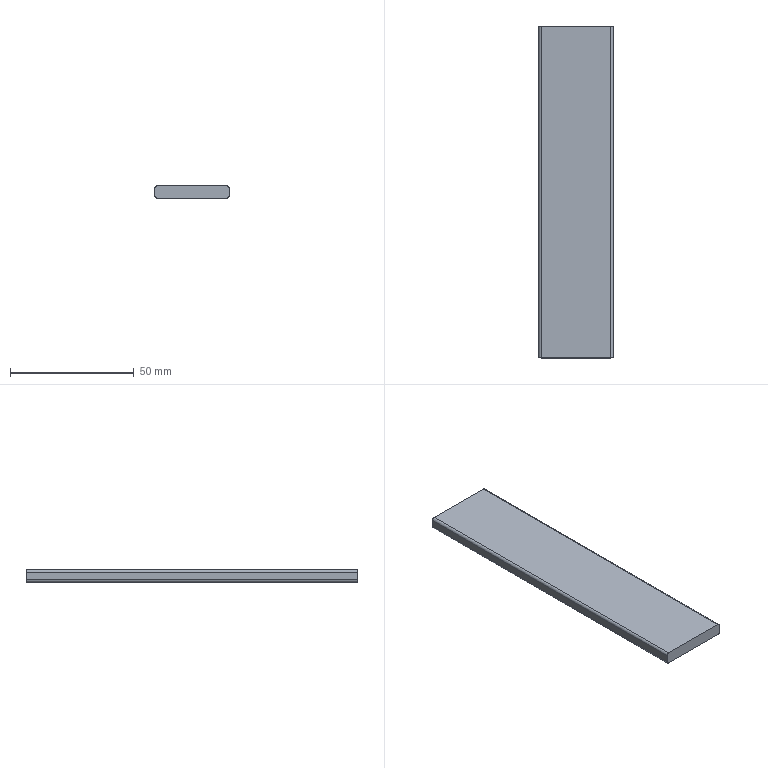Part | STEP file | Tube necking machine_id734_x_t | 1 solid | 10 faces | box 30 x 134 x 5 mm | volume 19985 mm3 | plane 6 | cylinder 4 | commonest cylinder face diameters 2 x4
STEP:
#1=CARTESIAN_POINT('',(0.,0.,0.));
#2=DIRECTION('',(0.,0.,1.));
#3=DIRECTION('',(1.,0.,0.));
#4=AXIS2_PLACEMENT_3D('',#1,#2,#3);
#5=CARTESIAN_POINT('',(-46.,-259.,196.));
#6=VERTEX_POINT('',#5);
#7=CARTESIAN_POINT('',(-74.,-259.,196.));
#8=VERTEX_POINT('',#7);
#9=CARTESIAN_POINT('',(-40.,-259.,196.));
#10=DIRECTION('',(-1.,0.,0.));
#11=VECTOR('',#10,1.);
#12=LINE('',#9,#11);
#13=CARTESIAN_POINT('',(-40.,-259.,196.));
#14=DIRECTION('',(0.,0.,-1.));
#15=DIRECTION('',(-1.,0.,0.));
#16=AXIS2_PLACEMENT_3D('',#13,#14,#15);
#17=PLANE('',#16);
#18=CARTESIAN_POINT('',(0.,0.));
#19=DIRECTION('',(1.,0.));
#20=VECTOR('',#19,1.);
#21=LINE('',#18,#20);
#22=(GEOMETRIC_REPRESENTATION_CONTEXT(2)PARAMETRIC_REPRESENTATION_CONTEXT()REPRESENTATION_CONTEXT('',''));
#23=DEFINITIONAL_REPRESENTATION('',(#21),#22);
#24=PCURVE('',#17,#23);
#25=CARTESIAN_POINT('',(0.,-259.,0.));
#26=DIRECTION('',(0.,-1.,0.));
#27=DIRECTION('',(0.,0.,-1.));
#28=AXIS2_PLACEMENT_3D('',#25,#26,#27);
#29=PLANE('',#28);
#30=CARTESIAN_POINT('',(-196.,-40.));
#31=DIRECTION('',(0.,-1.));
#32=VECTOR('',#31,1.);
#33=LINE('',#30,#32);
#34=(GEOMETRIC_REPRESENTATION_CONTEXT(2)PARAMETRIC_REPRESENTATION_CONTEXT()REPRESENTATION_CONTEXT('',''));
#35=DEFINITIONAL_REPRESENTATION('',(#33),#34);
#36=PCURVE('',#29,#35);
#37=SURFACE_CURVE('',#12,(#24,#36),.PCURVE_S1.);
#38=EDGE_CURVE('',#6,#8,#37,.T.);
#39=ORIENTED_EDGE('',*,*,#38,.F.);
#40=CARTESIAN_POINT('',(-46.,-125.,196.));
#41=VERTEX_POINT('',#40);
#42=CARTESIAN_POINT('',(-46.,-259.,196.));
#43=DIRECTION('',(0.,1.,0.));
#44=VECTOR('',#43,1.);
#45=LINE('',#42,#44);
#46=CARTESIAN_POINT('',(6.,0.));
#47=DIRECTION('',(0.,1.));
#48=VECTOR('',#47,1.);
#49=LINE('',#46,#48);
#50=(GEOMETRIC_REPRESENTATION_CONTEXT(2)PARAMETRIC_REPRESENTATION_CONTEXT()REPRESENTATION_CONTEXT('',''));
#51=DEFINITIONAL_REPRESENTATION('',(#49),#50);
#52=PCURVE('',#17,#51);
#53=CARTESIAN_POINT('',(-46.,-259.,195.));
#54=DIRECTION('',(0.,1.,0.));
#55=DIRECTION('',(0.,0.,1.));
#56=AXIS2_PLACEMENT_3D('',#53,#54,#55);
#57=CYLINDRICAL_SURFACE('',#56,1.);
#58=CARTESIAN_POINT('',(0.,0.));
#59=DIRECTION('',(0.,1.));
#60=VECTOR('',#59,1.);
#61=LINE('',#58,#60);
#62=(GEOMETRIC_REPRESENTATION_CONTEXT(2)PARAMETRIC_REPRESENTATION_CONTEXT()REPRESENTATION_CONTEXT('',''));
#63=DEFINITIONAL_REPRESENTATION('',(#61),#62);
#64=PCURVE('',#57,#63);
#65=SURFACE_CURVE('',#45,(#52,#64),.PCURVE_S1.);
#66=EDGE_CURVE('',#6,#41,#65,.T.);
#67=ORIENTED_EDGE('',*,*,#66,.T.);
#68=CARTESIAN_POINT('',(-74.,-125.,196.));
#69=VERTEX_POINT('',#68);
#70=CARTESIAN_POINT('',(-40.,-125.,196.));
#71=DIRECTION('',(-1.,0.,0.));
#72=VECTOR('',#71,1.);
#73=LINE('',#70,#72);
#74=CARTESIAN_POINT('',(0.,134.));
#75=DIRECTION('',(1.,0.));
#76=VECTOR('',#75,1.);
#77=LINE('',#74,#76);
#78=(GEOMETRIC_REPRESENTATION_CONTEXT(2)PARAMETRIC_REPRESENTATION_CONTEXT()REPRESENTATION_CONTEXT('',''));
#79=DEFINITIONAL_REPRESENTATION('',(#77),#78);
#80=PCURVE('',#17,#79);
#81=CARTESIAN_POINT('',(0.,-125.,0.));
#82=DIRECTION('',(0.,-1.,0.));
#83=DIRECTION('',(0.,0.,-1.));
#84=AXIS2_PLACEMENT_3D('',#81,#82,#83);
#85=PLANE('',#84);
#86=CARTESIAN_POINT('',(-196.,-40.));
#87=DIRECTION('',(0.,-1.));
#88=VECTOR('',#87,1.);
#89=LINE('',#86,#88);
#90=(GEOMETRIC_REPRESENTATION_CONTEXT(2)PARAMETRIC_REPRESENTATION_CONTEXT()REPRESENTATION_CONTEXT('',''));
#91=DEFINITIONAL_REPRESENTATION('',(#89),#90);
#92=PCURVE('',#85,#91);
#93=SURFACE_CURVE('',#73,(#80,#92),.PCURVE_S1.);
#94=EDGE_CURVE('',#41,#69,#93,.T.);
#95=ORIENTED_EDGE('',*,*,#94,.T.);
#96=CARTESIAN_POINT('',(-74.,-259.,196.));
#97=DIRECTION('',(0.,-1.,0.));
#98=VECTOR('',#97,1.);
#99=LINE('',#96,#98);
#100=CARTESIAN_POINT('',(34.,0.));
#101=DIRECTION('',(0.,-1.));
#102=VECTOR('',#101,1.);
#103=LINE('',#100,#102);
#104=(GEOMETRIC_REPRESENTATION_CONTEXT(2)PARAMETRIC_REPRESENTATION_CONTEXT()REPRESENTATION_CONTEXT('',''));
#105=DEFINITIONAL_REPRESENTATION('',(#103),#104);
#106=PCURVE('',#17,#105);
#107=CARTESIAN_POINT('',(-74.,-259.,195.));
#108=DIRECTION('',(0.,1.,0.));
#109=DIRECTION('',(0.,0.,1.));
#110=AXIS2_PLACEMENT_3D('',#107,#108,#109);
#111=CYLINDRICAL_SURFACE('',#110,1.);
#112=CARTESIAN_POINT('',(6.283,0.));
#113=DIRECTION('',(0.,-1.));
#114=VECTOR('',#113,1.);
#115=LINE('',#112,#114);
#116=(GEOMETRIC_REPRESENTATION_CONTEXT(2)PARAMETRIC_REPRESENTATION_CONTEXT()REPRESENTATION_CONTEXT('',''));
#117=DEFINITIONAL_REPRESENTATION('',(#115),#116);
#118=PCURVE('',#111,#117);
#119=SURFACE_CURVE('',#99,(#106,#118),.PCURVE_S1.);
#120=EDGE_CURVE('',#69,#8,#119,.T.);
#121=ORIENTED_EDGE('',*,*,#120,.T.);
#122=EDGE_LOOP('',(#39,#67,#95,#121));
#123=FACE_BOUND('',#122,.T.);
#124=ADVANCED_FACE('',(#123),#17,.F.);
#125=CARTESIAN_POINT('',(-75.,-125.,195.));
#126=VERTEX_POINT('',#125);
#127=CARTESIAN_POINT('',(-75.,-125.,192.));
#128=VERTEX_POINT('',#127);
#129=CARTESIAN_POINT('',(-75.,-125.,196.));
#130=DIRECTION('',(0.,0.,-1.));
#131=VECTOR('',#130,1.);
#132=LINE('',#129,#131);
#133=CARTESIAN_POINT('',(-75.,-259.,196.));
#134=DIRECTION('',(1.,0.,0.));
#135=DIRECTION('',(0.,0.,-1.));
#136=AXIS2_PLACEMENT_3D('',#133,#134,#135);
#137=PLANE('',#136);
#138=CARTESIAN_POINT('',(0.,134.));
#139=DIRECTION('',(1.,0.));
#140=VECTOR('',#139,1.);
#141=LINE('',#138,#140);
#142=(GEOMETRIC_REPRESENTATION_CONTEXT(2)PARAMETRIC_REPRESENTATION_CONTEXT()REPRESENTATION_CONTEXT('',''));
#143=DEFINITIONAL_REPRESENTATION('',(#141),#142);
#144=PCURVE('',#137,#143);
#145=CARTESIAN_POINT('',(-196.,-75.));
#146=DIRECTION('',(1.,0.));
#147=VECTOR('',#146,1.);
#148=LINE('',#145,#147);
#149=(GEOMETRIC_REPRESENTATION_CONTEXT(2)PARAMETRIC_REPRESENTATION_CONTEXT()REPRESENTATION_CONTEXT('',''));
#150=DEFINITIONAL_REPRESENTATION('',(#148),#149);
#151=PCURVE('',#85,#150);
#152=SURFACE_CURVE('',#132,(#144,#151),.PCURVE_S1.);
#153=EDGE_CURVE('',#126,#128,#152,.T.);
#154=ORIENTED_EDGE('',*,*,#153,.T.);
#155=CARTESIAN_POINT('',(-75.,-259.,192.));
#156=VERTEX_POINT('',#155);
#157=CARTESIAN_POINT('',(-75.,-259.,192.));
#158=DIRECTION('',(0.,-1.,0.));
#159=VECTOR('',#158,1.);
#160=LINE('',#157,#159);
#161=CARTESIAN_POINT('',(4.,0.));
#162=DIRECTION('',(0.,-1.));
#163=VECTOR('',#162,1.);
#164=LINE('',#161,#163);
#165=(GEOMETRIC_REPRESENTATION_CONTEXT(2)PARAMETRIC_REPRESENTATION_CONTEXT()REPRESENTATION_CONTEXT('',''));
#166=DEFINITIONAL_REPRESENTATION('',(#164),#165);
#167=PCURVE('',#137,#166);
#168=CARTESIAN_POINT('',(-74.,-259.,192.));
#169=DIRECTION('',(0.,1.,0.));
#170=DIRECTION('',(0.,0.,1.));
#171=AXIS2_PLACEMENT_3D('',#168,#169,#170);
#172=CYLINDRICAL_SURFACE('',#171,1.);
#173=CARTESIAN_POINT('',(4.712,0.));
#174=DIRECTION('',(0.,-1.));
#175=VECTOR('',#174,1.);
#176=LINE('',#173,#175);
#177=(GEOMETRIC_REPRESENTATION_CONTEXT(2)PARAMETRIC_REPRESENTATION_CONTEXT()REPRESENTATION_CONTEXT('',''));
#178=DEFINITIONAL_REPRESENTATION('',(#176),#177);
#179=PCURVE('',#172,#178);
#180=SURFACE_CURVE('',#160,(#167,#179),.PCURVE_S1.);
#181=EDGE_CURVE('',#128,#156,#180,.T.);
#182=ORIENTED_EDGE('',*,*,#181,.T.);
#183=CARTESIAN_POINT('',(-75.,-259.,195.));
#184=VERTEX_POINT('',#183);
#185=CARTESIAN_POINT('',(-75.,-259.,196.));
#186=DIRECTION('',(0.,0.,-1.));
#187=VECTOR('',#186,1.);
#188=LINE('',#185,#187);
#189=CARTESIAN_POINT('',(0.,0.));
#190=DIRECTION('',(1.,0.));
#191=VECTOR('',#190,1.);
#192=LINE('',#189,#191);
#193=(GEOMETRIC_REPRESENTATION_CONTEXT(2)PARAMETRIC_REPRESENTATION_CONTEXT()REPRESENTATION_CONTEXT('',''));
#194=DEFINITIONAL_REPRESENTATION('',(#192),#193);
#195=PCURVE('',#137,#194);
#196=CARTESIAN_POINT('',(-196.,-75.));
#197=DIRECTION('',(1.,0.));
#198=VECTOR('',#197,1.);
#199=LINE('',#196,#198);
#200=(GEOMETRIC_REPRESENTATION_CONTEXT(2)PARAMETRIC_REPRESENTATION_CONTEXT()REPRESENTATION_CONTEXT('',''));
#201=DEFINITIONAL_REPRESENTATION('',(#199),#200);
#202=PCURVE('',#29,#201);
#203=SURFACE_CURVE('',#188,(#195,#202),.PCURVE_S1.);
#204=EDGE_CURVE('',#184,#156,#203,.T.);
#205=ORIENTED_EDGE('',*,*,#204,.F.);
#206=CARTESIAN_POINT('',(-75.,-259.,195.));
#207=DIRECTION('',(0.,1.,0.));
#208=VECTOR('',#207,1.);
#209=LINE('',#206,#208);
#210=CARTESIAN_POINT('',(1.,0.));
#211=DIRECTION('',(0.,1.));
#212=VECTOR('',#211,1.);
#213=LINE('',#210,#212);
#214=(GEOMETRIC_REPRESENTATION_CONTEXT(2)PARAMETRIC_REPRESENTATION_CONTEXT()REPRESENTATION_CONTEXT('',''));
#215=DEFINITIONAL_REPRESENTATION('',(#213),#214);
#216=PCURVE('',#137,#215);
#217=CARTESIAN_POINT('',(4.712,0.));
#218=DIRECTION('',(0.,1.));
#219=VECTOR('',#218,1.);
#220=LINE('',#217,#219);
#221=(GEOMETRIC_REPRESENTATION_CONTEXT(2)PARAMETRIC_REPRESENTATION_CONTEXT()REPRESENTATION_CONTEXT('',''));
#222=DEFINITIONAL_REPRESENTATION('',(#220),#221);
#223=PCURVE('',#111,#222);
#224=SURFACE_CURVE('',#209,(#216,#223),.PCURVE_S1.);
#225=EDGE_CURVE('',#184,#126,#224,.T.);
#226=ORIENTED_EDGE('',*,*,#225,.T.);
#227=EDGE_LOOP('',(#154,#182,#205,#226));
#228=FACE_BOUND('',#227,.T.);
#229=ADVANCED_FACE('',(#228),#137,.F.);
#230=CARTESIAN_POINT('',(-74.,-125.,191.));
#231=VERTEX_POINT('',#230);
#232=CARTESIAN_POINT('',(-46.,-125.,191.));
#233=VERTEX_POINT('',#232);
#234=CARTESIAN_POINT('',(-75.,-125.,191.));
#235=DIRECTION('',(1.,0.,0.));
#236=VECTOR('',#235,1.);
#237=LINE('',#234,#236);
#238=CARTESIAN_POINT('',(-75.,-259.,191.));
#239=DIRECTION('',(0.,0.,1.));
#240=DIRECTION('',(1.,0.,0.));
#241=AXIS2_PLACEMENT_3D('',#238,#239,#240);
#242=PLANE('',#241);
#243=CARTESIAN_POINT('',(0.,134.));
#244=DIRECTION('',(1.,0.));
#245=VECTOR('',#244,1.);
#246=LINE('',#243,#245);
#247=(GEOMETRIC_REPRESENTATION_CONTEXT(2)PARAMETRIC_REPRESENTATION_CONTEXT()REPRESENTATION_CONTEXT('',''));
#248=DEFINITIONAL_REPRESENTATION('',(#246),#247);
#249=PCURVE('',#242,#248);
#250=CARTESIAN_POINT('',(-191.,-75.));
#251=DIRECTION('',(0.,1.));
#252=VECTOR('',#251,1.);
#253=LINE('',#250,#252);
#254=(GEOMETRIC_REPRESENTATION_CONTEXT(2)PARAMETRIC_REPRESENTATION_CONTEXT()REPRESENTATION_CONTEXT('',''));
#255=DEFINITIONAL_REPRESENTATION('',(#253),#254);
#256=PCURVE('',#85,#255);
#257=SURFACE_CURVE('',#237,(#249,#256),.PCURVE_S1.);
#258=EDGE_CURVE('',#231,#233,#257,.T.);
#259=ORIENTED_EDGE('',*,*,#258,.T.);
#260=CARTESIAN_POINT('',(-46.,-259.,191.));
#261=VERTEX_POINT('',#260);
#262=CARTESIAN_POINT('',(-46.,-259.,191.));
#263=DIRECTION('',(0.,-1.,0.));
#264=VECTOR('',#263,1.);
#265=LINE('',#262,#264);
#266=CARTESIAN_POINT('',(29.,0.));
#267=DIRECTION('',(0.,-1.));
#268=VECTOR('',#267,1.);
#269=LINE('',#266,#268);
#270=(GEOMETRIC_REPRESENTATION_CONTEXT(2)PARAMETRIC_REPRESENTATION_CONTEXT()REPRESENTATION_CONTEXT('',''));
#271=DEFINITIONAL_REPRESENTATION('',(#269),#270);
#272=PCURVE('',#242,#271);
#273=CARTESIAN_POINT('',(-46.,-259.,192.));
#274=DIRECTION('',(0.,1.,0.));
#275=DIRECTION('',(0.,0.,1.));
#276=AXIS2_PLACEMENT_3D('',#273,#274,#275);
#277=CYLINDRICAL_SURFACE('',#276,1.);
#278=CARTESIAN_POINT('',(3.142,0.));
#279=DIRECTION('',(0.,-1.));
#280=VECTOR('',#279,1.);
#281=LINE('',#278,#280);
#282=(GEOMETRIC_REPRESENTATION_CONTEXT(2)PARAMETRIC_REPRESENTATION_CONTEXT()REPRESENTATION_CONTEXT('',''));
#283=DEFINITIONAL_REPRESENTATION('',(#281),#282);
#284=PCURVE('',#277,#283);
#285=SURFACE_CURVE('',#265,(#272,#284),.PCURVE_S1.);
#286=EDGE_CURVE('',#233,#261,#285,.T.);
#287=ORIENTED_EDGE('',*,*,#286,.T.);
#288=CARTESIAN_POINT('',(-74.,-259.,191.));
#289=VERTEX_POINT('',#288);
#290=CARTESIAN_POINT('',(-75.,-259.,191.));
#291=DIRECTION('',(1.,0.,0.));
#292=VECTOR('',#291,1.);
#293=LINE('',#290,#292);
#294=CARTESIAN_POINT('',(0.,0.));
#295=DIRECTION('',(1.,0.));
#296=VECTOR('',#295,1.);
#297=LINE('',#294,#296);
#298=(GEOMETRIC_REPRESENTATION_CONTEXT(2)PARAMETRIC_REPRESENTATION_CONTEXT()REPRESENTATION_CONTEXT('',''));
#299=DEFINITIONAL_REPRESENTATION('',(#297),#298);
#300=PCURVE('',#242,#299);
#301=CARTESIAN_POINT('',(-191.,-75.));
#302=DIRECTION('',(0.,1.));
#303=VECTOR('',#302,1.);
#304=LINE('',#301,#303);
#305=(GEOMETRIC_REPRESENTATION_CONTEXT(2)PARAMETRIC_REPRESENTATION_CONTEXT()REPRESENTATION_CONTEXT('',''));
#306=DEFINITIONAL_REPRESENTATION('',(#304),#305);
#307=PCURVE('',#29,#306);
#308=SURFACE_CURVE('',#293,(#300,#307),.PCURVE_S1.);
#309=EDGE_CURVE('',#289,#261,#308,.T.);
#310=ORIENTED_EDGE('',*,*,#309,.F.);
#311=CARTESIAN_POINT('',(-74.,-259.,191.));
#312=DIRECTION('',(0.,1.,0.));
#313=VECTOR('',#312,1.);
#314=LINE('',#311,#313);
#315=CARTESIAN_POINT('',(1.,0.));
#316=DIRECTION('',(0.,1.));
#317=VECTOR('',#316,1.);
#318=LINE('',#315,#317);
#319=(GEOMETRIC_REPRESENTATION_CONTEXT(2)PARAMETRIC_REPRESENTATION_CONTEXT()REPRESENTATION_CONTEXT('',''));
#320=DEFINITIONAL_REPRESENTATION('',(#318),#319);
#321=PCURVE('',#242,#320);
#322=CARTESIAN_POINT('',(3.142,0.));
#323=DIRECTION('',(0.,1.));
#324=VECTOR('',#323,1.);
#325=LINE('',#322,#324);
#326=(GEOMETRIC_REPRESENTATION_CONTEXT(2)PARAMETRIC_REPRESENTATION_CONTEXT()REPRESENTATION_CONTEXT('',''));
#327=DEFINITIONAL_REPRESENTATION('',(#325),#326);
#328=PCURVE('',#172,#327);
#329=SURFACE_CURVE('',#314,(#321,#328),.PCURVE_S1.);
#330=EDGE_CURVE('',#289,#231,#329,.T.);
#331=ORIENTED_EDGE('',*,*,#330,.T.);
#332=EDGE_LOOP('',(#259,#287,#310,#331));
#333=FACE_BOUND('',#332,.T.);
#334=ADVANCED_FACE('',(#333),#242,.F.);
#335=CARTESIAN_POINT('',(-45.,-259.,192.));
#336=VERTEX_POINT('',#335);
#337=CARTESIAN_POINT('',(-45.,-259.,195.));
#338=VERTEX_POINT('',#337);
#339=CARTESIAN_POINT('',(-45.,-259.,191.));
#340=DIRECTION('',(0.,0.,1.));
#341=VECTOR('',#340,1.);
#342=LINE('',#339,#341);
#343=CARTESIAN_POINT('',(-45.,-259.,191.));
#344=DIRECTION('',(-1.,0.,0.));
#345=DIRECTION('',(0.,0.,1.));
#346=AXIS2_PLACEMENT_3D('',#343,#344,#345);
#347=PLANE('',#346);
#348=CARTESIAN_POINT('',(0.,0.));
#349=DIRECTION('',(1.,0.));
#350=VECTOR('',#349,1.);
#351=LINE('',#348,#350);
#352=(GEOMETRIC_REPRESENTATION_CONTEXT(2)PARAMETRIC_REPRESENTATION_CONTEXT()REPRESENTATION_CONTEXT('',''));
#353=DEFINITIONAL_REPRESENTATION('',(#351),#352);
#354=PCURVE('',#347,#353);
#355=CARTESIAN_POINT('',(-191.,-45.));
#356=DIRECTION('',(-1.,0.));
#357=VECTOR('',#356,1.);
#358=LINE('',#355,#357);
#359=(GEOMETRIC_REPRESENTATION_CONTEXT(2)PARAMETRIC_REPRESENTATION_CONTEXT()REPRESENTATION_CONTEXT('',''));
#360=DEFINITIONAL_REPRESENTATION('',(#358),#359);
#361=PCURVE('',#29,#360);
#362=SURFACE_CURVE('',#342,(#354,#361),.PCURVE_S1.);
#363=EDGE_CURVE('',#336,#338,#362,.T.);
#364=ORIENTED_EDGE('',*,*,#363,.F.);
#365=CARTESIAN_POINT('',(-45.,-125.,192.));
#366=VERTEX_POINT('',#365);
#367=CARTESIAN_POINT('',(-45.,-259.,192.));
#368=DIRECTION('',(0.,1.,0.));
#369=VECTOR('',#368,1.);
#370=LINE('',#367,#369);
#371=CARTESIAN_POINT('',(1.,0.));
#372=DIRECTION('',(0.,1.));
#373=VECTOR('',#372,1.);
#374=LINE('',#371,#373);
#375=(GEOMETRIC_REPRESENTATION_CONTEXT(2)PARAMETRIC_REPRESENTATION_CONTEXT()REPRESENTATION_CONTEXT('',''));
#376=DEFINITIONAL_REPRESENTATION('',(#374),#375);
#377=PCURVE('',#347,#376);
#378=CARTESIAN_POINT('',(1.571,0.));
#379=DIRECTION('',(0.,1.));
#380=VECTOR('',#379,1.);
#381=LINE('',#378,#380);
#382=(GEOMETRIC_REPRESENTATION_CONTEXT(2)PARAMETRIC_REPRESENTATION_CONTEXT()REPRESENTATION_CONTEXT('',''));
#383=DEFINITIONAL_REPRESENTATION('',(#381),#382);
#384=PCURVE('',#277,#383);
#385=SURFACE_CURVE('',#370,(#377,#384),.PCURVE_S1.);
#386=EDGE_CURVE('',#336,#366,#385,.T.);
#387=ORIENTED_EDGE('',*,*,#386,.T.);
#388=CARTESIAN_POINT('',(-45.,-125.,195.));
#389=VERTEX_POINT('',#388);
#390=CARTESIAN_POINT('',(-45.,-125.,191.));
#391=DIRECTION('',(0.,0.,1.));
#392=VECTOR('',#391,1.);
#393=LINE('',#390,#392);
#394=CARTESIAN_POINT('',(0.,134.));
#395=DIRECTION('',(1.,0.));
#396=VECTOR('',#395,1.);
#397=LINE('',#394,#396);
#398=(GEOMETRIC_REPRESENTATION_CONTEXT(2)PARAMETRIC_REPRESENTATION_CONTEXT()REPRESENTATION_CONTEXT('',''));
#399=DEFINITIONAL_REPRESENTATION('',(#397),#398);
#400=PCURVE('',#347,#399);
#401=CARTESIAN_POINT('',(-191.,-45.));
#402=DIRECTION('',(-1.,0.));
#403=VECTOR('',#402,1.);
#404=LINE('',#401,#403);
#405=(GEOMETRIC_REPRESENTATION_CONTEXT(2)PARAMETRIC_REPRESENTATION_CONTEXT()REPRESENTATION_CONTEXT('',''));
#406=DEFINITIONAL_REPRESENTATION('',(#404),#405);
#407=PCURVE('',#85,#406);
#408=SURFACE_CURVE('',#393,(#400,#407),.PCURVE_S1.);
#409=EDGE_CURVE('',#366,#389,#408,.T.);
#410=ORIENTED_EDGE('',*,*,#409,.T.);
#411=CARTESIAN_POINT('',(-45.,-259.,195.));
#412=DIRECTION('',(0.,-1.,0.));
#413=VECTOR('',#412,1.);
#414=LINE('',#411,#413);
#415=CARTESIAN_POINT('',(4.,0.));
#416=DIRECTION('',(0.,-1.));
#417=VECTOR('',#416,1.);
#418=LINE('',#415,#417);
#419=(GEOMETRIC_REPRESENTATION_CONTEXT(2)PARAMETRIC_REPRESENTATION_CONTEXT()REPRESENTATION_CONTEXT('',''));
#420=DEFINITIONAL_REPRESENTATION('',(#418),#419);
#421=PCURVE('',#347,#420);
#422=CARTESIAN_POINT('',(1.571,0.));
#423=DIRECTION('',(0.,-1.));
#424=VECTOR('',#423,1.);
#425=LINE('',#422,#424);
#426=(GEOMETRIC_REPRESENTATION_CONTEXT(2)PARAMETRIC_REPRESENTATION_CONTEXT()REPRESENTATION_CONTEXT('',''));
#427=DEFINITIONAL_REPRESENTATION('',(#425),#426);
#428=PCURVE('',#57,#427);
#429=SURFACE_CURVE('',#414,(#421,#428),.PCURVE_S1.);
#430=EDGE_CURVE('',#389,#338,#429,.T.);
#431=ORIENTED_EDGE('',*,*,#430,.T.);
#432=EDGE_LOOP('',(#364,#387,#410,#431));
#433=FACE_BOUND('',#432,.T.);
#434=ADVANCED_FACE('',(#433),#347,.F.);
#435=ORIENTED_EDGE('',*,*,#309,.T.);
#436=CARTESIAN_POINT('',(-46.,-259.,192.));
#437=DIRECTION('',(0.,-1.,0.));
#438=DIRECTION('',(0.,0.,-1.));
#439=AXIS2_PLACEMENT_3D('',#436,#437,#438);
#440=CIRCLE('',#439,1.);
#441=CARTESIAN_POINT('',(-192.,-46.));
#442=DIRECTION('',(1.,0.));
#443=AXIS2_PLACEMENT_2D('',#441,#442);
#444=CIRCLE('',#443,1.);
#445=(GEOMETRIC_REPRESENTATION_CONTEXT(2)PARAMETRIC_REPRESENTATION_CONTEXT()REPRESENTATION_CONTEXT('',''));
#446=DEFINITIONAL_REPRESENTATION('',(#444),#445);
#447=PCURVE('',#29,#446);
#448=CARTESIAN_POINT('',(3.142,0.));
#449=DIRECTION('',(-1.,0.));
#450=VECTOR('',#449,1.);
#451=LINE('',#448,#450);
#452=(GEOMETRIC_REPRESENTATION_CONTEXT(2)PARAMETRIC_REPRESENTATION_CONTEXT()REPRESENTATION_CONTEXT('',''));
#453=DEFINITIONAL_REPRESENTATION('',(#451),#452);
#454=PCURVE('',#277,#453);
#455=SURFACE_CURVE('',#440,(#447,#454),.PCURVE_S1.);
#456=EDGE_CURVE('',#261,#336,#455,.T.);
#457=ORIENTED_EDGE('',*,*,#456,.T.);
#458=ORIENTED_EDGE('',*,*,#363,.T.);
#459=CARTESIAN_POINT('',(-46.,-259.,195.));
#460=DIRECTION('',(0.,-1.,0.));
#461=DIRECTION('',(0.,0.,-1.));
#462=AXIS2_PLACEMENT_3D('',#459,#460,#461);
#463=CIRCLE('',#462,1.);
#464=CARTESIAN_POINT('',(-195.,-46.));
#465=DIRECTION('',(1.,0.));
#466=AXIS2_PLACEMENT_2D('',#464,#465);
#467=CIRCLE('',#466,1.);
#468=(GEOMETRIC_REPRESENTATION_CONTEXT(2)PARAMETRIC_REPRESENTATION_CONTEXT()REPRESENTATION_CONTEXT('',''));
#469=DEFINITIONAL_REPRESENTATION('',(#467),#468);
#470=PCURVE('',#29,#469);
#471=CARTESIAN_POINT('',(3.142,0.));
#472=DIRECTION('',(-1.,0.));
#473=VECTOR('',#472,1.);
#474=LINE('',#471,#473);
#475=(GEOMETRIC_REPRESENTATION_CONTEXT(2)PARAMETRIC_REPRESENTATION_CONTEXT()REPRESENTATION_CONTEXT('',''));
#476=DEFINITIONAL_REPRESENTATION('',(#474),#475);
#477=PCURVE('',#57,#476);
#478=SURFACE_CURVE('',#463,(#470,#477),.PCURVE_S1.);
#479=EDGE_CURVE('',#338,#6,#478,.T.);
#480=ORIENTED_EDGE('',*,*,#479,.T.);
#481=ORIENTED_EDGE('',*,*,#38,.T.);
#482=CARTESIAN_POINT('',(-74.,-259.,195.));
#483=DIRECTION('',(0.,-1.,0.));
#484=DIRECTION('',(0.,0.,-1.));
#485=AXIS2_PLACEMENT_3D('',#482,#483,#484);
#486=CIRCLE('',#485,1.);
#487=CARTESIAN_POINT('',(-195.,-74.));
#488=DIRECTION('',(1.,0.));
#489=AXIS2_PLACEMENT_2D('',#487,#488);
#490=CIRCLE('',#489,1.);
#491=(GEOMETRIC_REPRESENTATION_CONTEXT(2)PARAMETRIC_REPRESENTATION_CONTEXT()REPRESENTATION_CONTEXT('',''));
#492=DEFINITIONAL_REPRESENTATION('',(#490),#491);
#493=PCURVE('',#29,#492);
#494=CARTESIAN_POINT('',(9.425,0.));
#495=DIRECTION('',(-1.,0.));
#496=VECTOR('',#495,1.);
#497=LINE('',#494,#496);
#498=(GEOMETRIC_REPRESENTATION_CONTEXT(2)PARAMETRIC_REPRESENTATION_CONTEXT()REPRESENTATION_CONTEXT('',''));
#499=DEFINITIONAL_REPRESENTATION('',(#497),#498);
#500=PCURVE('',#111,#499);
#501=SURFACE_CURVE('',#486,(#493,#500),.PCURVE_S1.);
#502=EDGE_CURVE('',#8,#184,#501,.T.);
#503=ORIENTED_EDGE('',*,*,#502,.T.);
#504=ORIENTED_EDGE('',*,*,#204,.T.);
#505=CARTESIAN_POINT('',(-74.,-259.,192.));
#506=DIRECTION('',(0.,-1.,0.));
#507=DIRECTION('',(0.,0.,-1.));
#508=AXIS2_PLACEMENT_3D('',#505,#506,#507);
#509=CIRCLE('',#508,1.);
#510=CARTESIAN_POINT('',(-192.,-74.));
#511=DIRECTION('',(1.,0.));
#512=AXIS2_PLACEMENT_2D('',#510,#511);
#513=CIRCLE('',#512,1.);
#514=(GEOMETRIC_REPRESENTATION_CONTEXT(2)PARAMETRIC_REPRESENTATION_CONTEXT()REPRESENTATION_CONTEXT('',''));
#515=DEFINITIONAL_REPRESENTATION('',(#513),#514);
#516=PCURVE('',#29,#515);
#517=CARTESIAN_POINT('',(9.425,0.));
#518=DIRECTION('',(-1.,0.));
#519=VECTOR('',#518,1.);
#520=LINE('',#517,#519);
#521=(GEOMETRIC_REPRESENTATION_CONTEXT(2)PARAMETRIC_REPRESENTATION_CONTEXT()REPRESENTATION_CONTEXT('',''));
#522=DEFINITIONAL_REPRESENTATION('',(#520),#521);
#523=PCURVE('',#172,#522);
#524=SURFACE_CURVE('',#509,(#516,#523),.PCURVE_S1.);
#525=EDGE_CURVE('',#156,#289,#524,.T.);
#526=ORIENTED_EDGE('',*,*,#525,.T.);
#527=EDGE_LOOP('',(#435,#457,#458,#480,#481,#503,#504,#526));
#528=FACE_BOUND('',#527,.T.);
#529=ADVANCED_FACE('',(#528),#29,.T.);
#530=ORIENTED_EDGE('',*,*,#409,.F.);
#531=CARTESIAN_POINT('',(-46.,-125.,192.));
#532=DIRECTION('',(0.,1.,0.));
#533=DIRECTION('',(0.,0.,-1.));
#534=AXIS2_PLACEMENT_3D('',#531,#532,#533);
#535=CIRCLE('',#534,1.);
#536=CARTESIAN_POINT('',(-191.,-46.));
#537=CARTESIAN_POINT('',(-191.,-47.732));
#538=CARTESIAN_POINT('',(-192.5,-46.866));
#539=CARTESIAN_POINT('',(-194.,-46.));
#540=CARTESIAN_POINT('',(-192.5,-45.134));
#541=CARTESIAN_POINT('',(-191.,-44.268));
#542=CARTESIAN_POINT('',(-191.,-46.));
#543=(BOUNDED_CURVE()B_SPLINE_CURVE(2,(#536,#537,#538,#539,#540,#541,#542),.UNSPECIFIED.,.T.,.F.)B_SPLINE_CURVE_WITH_KNOTS((1,2,2,2,2,1),(-2.094,0.,2.094,4.189,6.283,8.378),.UNSPECIFIED.)CURVE()GEOMETRIC_REPRESENTATION_ITEM()RATIONAL_B_SPLINE_CURVE((1.,0.5,1.,0.5,1.,0.5,1.))REPRESENTATION_ITEM(''));
#544=(GEOMETRIC_REPRESENTATION_CONTEXT(2)PARAMETRIC_REPRESENTATION_CONTEXT()REPRESENTATION_CONTEXT('',''));
#545=DEFINITIONAL_REPRESENTATION('',(#543),#544);
#546=PCURVE('',#85,#545);
#547=CARTESIAN_POINT('',(-3.142,134.));
#548=DIRECTION('',(1.,0.));
#549=VECTOR('',#548,1.);
#550=LINE('',#547,#549);
#551=(GEOMETRIC_REPRESENTATION_CONTEXT(2)PARAMETRIC_REPRESENTATION_CONTEXT()REPRESENTATION_CONTEXT('',''));
#552=DEFINITIONAL_REPRESENTATION('',(#550),#551);
#553=PCURVE('',#277,#552);
#554=SURFACE_CURVE('',#535,(#546,#553),.PCURVE_S1.);
#555=EDGE_CURVE('',#366,#233,#554,.T.);
#556=ORIENTED_EDGE('',*,*,#555,.T.);
#557=ORIENTED_EDGE('',*,*,#258,.F.);
#558=CARTESIAN_POINT('',(-74.,-125.,192.));
#559=DIRECTION('',(0.,1.,0.));
#560=DIRECTION('',(0.,0.,-1.));
#561=AXIS2_PLACEMENT_3D('',#558,#559,#560);
#562=CIRCLE('',#561,1.);
#563=CARTESIAN_POINT('',(-191.,-74.));
#564=CARTESIAN_POINT('',(-191.,-75.732));
#565=CARTESIAN_POINT('',(-192.5,-74.866));
#566=CARTESIAN_POINT('',(-194.,-74.));
#567=CARTESIAN_POINT('',(-192.5,-73.134));
#568=CARTESIAN_POINT('',(-191.,-72.268));
#569=CARTESIAN_POINT('',(-191.,-74.));
#570=(BOUNDED_CURVE()B_SPLINE_CURVE(2,(#563,#564,#565,#566,#567,#568,#569),.UNSPECIFIED.,.T.,.F.)B_SPLINE_CURVE_WITH_KNOTS((1,2,2,2,2,1),(-2.094,0.,2.094,4.189,6.283,8.378),.UNSPECIFIED.)CURVE()GEOMETRIC_REPRESENTATION_ITEM()RATIONAL_B_SPLINE_CURVE((1.,0.5,1.,0.5,1.,0.5,1.))REPRESENTATION_ITEM(''));
#571=(GEOMETRIC_REPRESENTATION_CONTEXT(2)PARAMETRIC_REPRESENTATION_CONTEXT()REPRESENTATION_CONTEXT('',''));
#572=DEFINITIONAL_REPRESENTATION('',(#570),#571);
#573=PCURVE('',#85,#572);
#574=CARTESIAN_POINT('',(3.142,134.));
#575=DIRECTION('',(1.,0.));
#576=VECTOR('',#575,1.);
#577=LINE('',#574,#576);
#578=(GEOMETRIC_REPRESENTATION_CONTEXT(2)PARAMETRIC_REPRESENTATION_CONTEXT()REPRESENTATION_CONTEXT('',''));
#579=DEFINITIONAL_REPRESENTATION('',(#577),#578);
#580=PCURVE('',#172,#579);
#581=SURFACE_CURVE('',#562,(#573,#580),.PCURVE_S1.);
#582=EDGE_CURVE('',#231,#128,#581,.T.);
#583=ORIENTED_EDGE('',*,*,#582,.T.);
#584=ORIENTED_EDGE('',*,*,#153,.F.);
#585=CARTESIAN_POINT('',(-74.,-125.,195.));
#586=DIRECTION('',(0.,1.,0.));
#587=DIRECTION('',(0.,0.,-1.));
#588=AXIS2_PLACEMENT_3D('',#585,#586,#587);
#589=CIRCLE('',#588,1.);
#590=CARTESIAN_POINT('',(-194.,-74.));
#591=CARTESIAN_POINT('',(-194.,-75.732));
#592=CARTESIAN_POINT('',(-195.5,-74.866));
#593=CARTESIAN_POINT('',(-197.,-74.));
#594=CARTESIAN_POINT('',(-195.5,-73.134));
#595=CARTESIAN_POINT('',(-194.,-72.268));
#596=CARTESIAN_POINT('',(-194.,-74.));
#597=(BOUNDED_CURVE()B_SPLINE_CURVE(2,(#590,#591,#592,#593,#594,#595,#596),.UNSPECIFIED.,.T.,.F.)B_SPLINE_CURVE_WITH_KNOTS((1,2,2,2,2,1),(-2.094,0.,2.094,4.189,6.283,8.378),.UNSPECIFIED.)CURVE()GEOMETRIC_REPRESENTATION_ITEM()RATIONAL_B_SPLINE_CURVE((1.,0.5,1.,0.5,1.,0.5,1.))REPRESENTATION_ITEM(''));
#598=(GEOMETRIC_REPRESENTATION_CONTEXT(2)PARAMETRIC_REPRESENTATION_CONTEXT()REPRESENTATION_CONTEXT('',''));
#599=DEFINITIONAL_REPRESENTATION('',(#597),#598);
#600=PCURVE('',#85,#599);
#601=CARTESIAN_POINT('',(3.142,134.));
#602=DIRECTION('',(1.,0.));
#603=VECTOR('',#602,1.);
#604=LINE('',#601,#603);
#605=(GEOMETRIC_REPRESENTATION_CONTEXT(2)PARAMETRIC_REPRESENTATION_CONTEXT()REPRESENTATION_CONTEXT('',''));
#606=DEFINITIONAL_REPRESENTATION('',(#604),#605);
#607=PCURVE('',#111,#606);
#608=SURFACE_CURVE('',#589,(#600,#607),.PCURVE_S1.);
#609=EDGE_CURVE('',#126,#69,#608,.T.);
#610=ORIENTED_EDGE('',*,*,#609,.T.);
#611=ORIENTED_EDGE('',*,*,#94,.F.);
#612=CARTESIAN_POINT('',(-46.,-125.,195.));
#613=DIRECTION('',(0.,1.,0.));
#614=DIRECTION('',(0.,0.,-1.));
#615=AXIS2_PLACEMENT_3D('',#612,#613,#614);
#616=CIRCLE('',#615,1.);
#617=CARTESIAN_POINT('',(-194.,-46.));
#618=CARTESIAN_POINT('',(-194.,-47.732));
#619=CARTESIAN_POINT('',(-195.5,-46.866));
#620=CARTESIAN_POINT('',(-197.,-46.));
#621=CARTESIAN_POINT('',(-195.5,-45.134));
#622=CARTESIAN_POINT('',(-194.,-44.268));
#623=CARTESIAN_POINT('',(-194.,-46.));
#624=(BOUNDED_CURVE()B_SPLINE_CURVE(2,(#617,#618,#619,#620,#621,#622,#623),.UNSPECIFIED.,.T.,.F.)B_SPLINE_CURVE_WITH_KNOTS((1,2,2,2,2,1),(-2.094,0.,2.094,4.189,6.283,8.378),.UNSPECIFIED.)CURVE()GEOMETRIC_REPRESENTATION_ITEM()RATIONAL_B_SPLINE_CURVE((1.,0.5,1.,0.5,1.,0.5,1.))REPRESENTATION_ITEM(''));
#625=(GEOMETRIC_REPRESENTATION_CONTEXT(2)PARAMETRIC_REPRESENTATION_CONTEXT()REPRESENTATION_CONTEXT('',''));
#626=DEFINITIONAL_REPRESENTATION('',(#624),#625);
#627=PCURVE('',#85,#626);
#628=CARTESIAN_POINT('',(-3.142,134.));
#629=DIRECTION('',(1.,0.));
#630=VECTOR('',#629,1.);
#631=LINE('',#628,#630);
#632=(GEOMETRIC_REPRESENTATION_CONTEXT(2)PARAMETRIC_REPRESENTATION_CONTEXT()REPRESENTATION_CONTEXT('',''));
#633=DEFINITIONAL_REPRESENTATION('',(#631),#632);
#634=PCURVE('',#57,#633);
#635=SURFACE_CURVE('',#616,(#627,#634),.PCURVE_S1.);
#636=EDGE_CURVE('',#41,#389,#635,.T.);
#637=ORIENTED_EDGE('',*,*,#636,.T.);
#638=EDGE_LOOP('',(#530,#556,#557,#583,#584,#610,#611,#637));
#639=FACE_BOUND('',#638,.T.);
#640=ADVANCED_FACE('',(#639),#85,.F.);
#641=ORIENTED_EDGE('',*,*,#456,.F.);
#642=ORIENTED_EDGE('',*,*,#286,.F.);
#643=ORIENTED_EDGE('',*,*,#555,.F.);
#644=ORIENTED_EDGE('',*,*,#386,.F.);
#645=EDGE_LOOP('',(#641,#642,#643,#644));
#646=FACE_BOUND('',#645,.T.);
#647=ADVANCED_FACE('',(#646),#277,.T.);
#648=ORIENTED_EDGE('',*,*,#479,.F.);
#649=ORIENTED_EDGE('',*,*,#430,.F.);
#650=ORIENTED_EDGE('',*,*,#636,.F.);
#651=ORIENTED_EDGE('',*,*,#66,.F.);
#652=EDGE_LOOP('',(#648,#649,#650,#651));
#653=FACE_BOUND('',#652,.T.);
#654=ADVANCED_FACE('',(#653),#57,.T.);
#655=ORIENTED_EDGE('',*,*,#525,.F.);
#656=ORIENTED_EDGE('',*,*,#181,.F.);
#657=ORIENTED_EDGE('',*,*,#582,.F.);
#658=ORIENTED_EDGE('',*,*,#330,.F.);
#659=EDGE_LOOP('',(#655,#656,#657,#658));
#660=FACE_BOUND('',#659,.T.);
#661=ADVANCED_FACE('',(#660),#172,.T.);
#662=ORIENTED_EDGE('',*,*,#502,.F.);
#663=ORIENTED_EDGE('',*,*,#120,.F.);
#664=ORIENTED_EDGE('',*,*,#609,.F.);
#665=ORIENTED_EDGE('',*,*,#225,.F.);
#666=EDGE_LOOP('',(#662,#663,#664,#665));
#667=FACE_BOUND('',#666,.T.);
#668=ADVANCED_FACE('',(#667),#111,.T.);
#669=CLOSED_SHELL('',(#124,#229,#334,#434,#529,#640,#647,#654,#661,#668));
#670=MANIFOLD_SOLID_BREP('',#669);
#671=(LENGTH_UNIT()NAMED_UNIT(*)SI_UNIT(.MILLI.,.METRE.));
#672=UNCERTAINTY_MEASURE_WITH_UNIT(LENGTH_MEASURE(0.0000001),#671,'','');
#673=(NAMED_UNIT(*)PLANE_ANGLE_UNIT()SI_UNIT($,.RADIAN.));
#674=(NAMED_UNIT(*)SI_UNIT($,.STERADIAN.)SOLID_ANGLE_UNIT());
#675=(GEOMETRIC_REPRESENTATION_CONTEXT(3)GLOBAL_UNCERTAINTY_ASSIGNED_CONTEXT((#672))GLOBAL_UNIT_ASSIGNED_CONTEXT((#671,#673,#674))REPRESENTATION_CONTEXT('',''));
#676=ADVANCED_BREP_SHAPE_REPRESENTATION('',(#4,#670),#675);